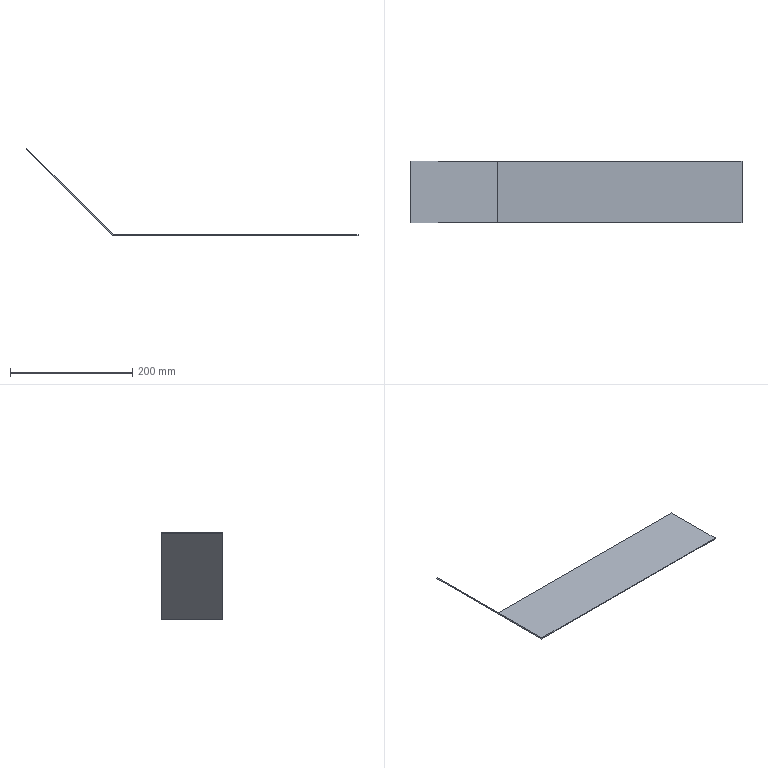Part | STEP file | Mirror Velcro | 1 solid | 8 faces | box 542.128 x 100 x 143.128 mm | volume 120000 mm3 | plane 8
STEP:
#1=CARTESIAN_POINT('',(0.,0.,0.));
#2=DIRECTION('',(0.,0.,1.));
#3=DIRECTION('',(1.,0.,0.));
#4=AXIS2_PLACEMENT_3D('',#1,#2,#3);
#5=CARTESIAN_POINT('',(-0.4142,-50.,-1.));
#6=VERTEX_POINT('',#5);
#7=CARTESIAN_POINT('',(400.,-50.,-1.));
#8=VERTEX_POINT('',#7);
#9=CARTESIAN_POINT('',(0.,-50.,-1.));
#10=DIRECTION('',(1.,0.,0.));
#11=VECTOR('',#10,1.);
#12=LINE('',#9,#11);
#13=CARTESIAN_POINT('',(0.,50.,-1.));
#14=DIRECTION('',(0.,0.,1.));
#15=DIRECTION('',(-1.,0.,0.));
#16=AXIS2_PLACEMENT_3D('',#13,#14,#15);
#17=PLANE('',#16);
#18=CARTESIAN_POINT('',(0.,100.));
#19=DIRECTION('',(-1.,0.));
#20=VECTOR('',#19,1.);
#21=LINE('',#18,#20);
#22=(GEOMETRIC_REPRESENTATION_CONTEXT(2)PARAMETRIC_REPRESENTATION_CONTEXT()REPRESENTATION_CONTEXT('',''));
#23=DEFINITIONAL_REPRESENTATION('',(#21),#22);
#24=PCURVE('',#17,#23);
#25=CARTESIAN_POINT('',(0.,-50.,0.));
#26=DIRECTION('',(0.,-1.,0.));
#27=DIRECTION('',(-1.,0.,0.));
#28=AXIS2_PLACEMENT_3D('',#25,#26,#27);
#29=PLANE('',#28);
#30=CARTESIAN_POINT('',(0.,1.));
#31=DIRECTION('',(-1.,0.));
#32=VECTOR('',#31,1.);
#33=LINE('',#30,#32);
#34=(GEOMETRIC_REPRESENTATION_CONTEXT(2)PARAMETRIC_REPRESENTATION_CONTEXT()REPRESENTATION_CONTEXT('',''));
#35=DEFINITIONAL_REPRESENTATION('',(#33),#34);
#36=PCURVE('',#29,#35);
#37=SURFACE_CURVE('',#12,(#24,#36),.PCURVE_S1.);
#38=EDGE_CURVE('',#6,#8,#37,.T.);
#39=ORIENTED_EDGE('',*,*,#38,.F.);
#40=CARTESIAN_POINT('',(-0.4142,50.,-1.));
#41=VERTEX_POINT('',#40);
#42=CARTESIAN_POINT('',(-0.4142,50.,-1.));
#43=DIRECTION('',(0.,-1.,0.));
#44=VECTOR('',#43,1.);
#45=LINE('',#42,#44);
#46=CARTESIAN_POINT('',(0.4142,0.));
#47=DIRECTION('',(0.,1.));
#48=VECTOR('',#47,1.);
#49=LINE('',#46,#48);
#50=(GEOMETRIC_REPRESENTATION_CONTEXT(2)PARAMETRIC_REPRESENTATION_CONTEXT()REPRESENTATION_CONTEXT('',''));
#51=DEFINITIONAL_REPRESENTATION('',(#49),#50);
#52=PCURVE('',#17,#51);
#53=CARTESIAN_POINT('',(-142.128,50.,140.714));
#54=DIRECTION('',(0.7071,0.,0.7071));
#55=DIRECTION('',(-0.7071,0.,0.7071));
#56=AXIS2_PLACEMENT_3D('',#53,#54,#55);
#57=PLANE('',#56);
#58=CARTESIAN_POINT('',(-200.414,0.));
#59=DIRECTION('',(0.,1.));
#60=VECTOR('',#59,1.);
#61=LINE('',#58,#60);
#62=(GEOMETRIC_REPRESENTATION_CONTEXT(2)PARAMETRIC_REPRESENTATION_CONTEXT()REPRESENTATION_CONTEXT('',''));
#63=DEFINITIONAL_REPRESENTATION('',(#61),#62);
#64=PCURVE('',#57,#63);
#65=SURFACE_CURVE('',#45,(#52,#64),.PCURVE_S1.);
#66=EDGE_CURVE('',#41,#6,#65,.T.);
#67=ORIENTED_EDGE('',*,*,#66,.F.);
#68=CARTESIAN_POINT('',(400.,50.,-1.));
#69=VERTEX_POINT('',#68);
#70=CARTESIAN_POINT('',(0.,50.,-1.));
#71=DIRECTION('',(1.,0.,0.));
#72=VECTOR('',#71,1.);
#73=LINE('',#70,#72);
#74=CARTESIAN_POINT('',(0.,0.));
#75=DIRECTION('',(-1.,0.));
#76=VECTOR('',#75,1.);
#77=LINE('',#74,#76);
#78=(GEOMETRIC_REPRESENTATION_CONTEXT(2)PARAMETRIC_REPRESENTATION_CONTEXT()REPRESENTATION_CONTEXT('',''));
#79=DEFINITIONAL_REPRESENTATION('',(#77),#78);
#80=PCURVE('',#17,#79);
#81=CARTESIAN_POINT('',(0.,50.,0.));
#82=DIRECTION('',(0.,-1.,0.));
#83=DIRECTION('',(-1.,0.,0.));
#84=AXIS2_PLACEMENT_3D('',#81,#82,#83);
#85=PLANE('',#84);
#86=CARTESIAN_POINT('',(0.,1.));
#87=DIRECTION('',(-1.,0.));
#88=VECTOR('',#87,1.);
#89=LINE('',#86,#88);
#90=(GEOMETRIC_REPRESENTATION_CONTEXT(2)PARAMETRIC_REPRESENTATION_CONTEXT()REPRESENTATION_CONTEXT('',''));
#91=DEFINITIONAL_REPRESENTATION('',(#89),#90);
#92=PCURVE('',#85,#91);
#93=SURFACE_CURVE('',#73,(#80,#92),.PCURVE_S1.);
#94=EDGE_CURVE('',#41,#69,#93,.T.);
#95=ORIENTED_EDGE('',*,*,#94,.T.);
#96=CARTESIAN_POINT('',(400.,50.,-1.));
#97=DIRECTION('',(0.,-1.,0.));
#98=VECTOR('',#97,1.);
#99=LINE('',#96,#98);
#100=CARTESIAN_POINT('',(-400.,0.));
#101=DIRECTION('',(0.,1.));
#102=VECTOR('',#101,1.);
#103=LINE('',#100,#102);
#104=(GEOMETRIC_REPRESENTATION_CONTEXT(2)PARAMETRIC_REPRESENTATION_CONTEXT()REPRESENTATION_CONTEXT('',''));
#105=DEFINITIONAL_REPRESENTATION('',(#103),#104);
#106=PCURVE('',#17,#105);
#107=CARTESIAN_POINT('',(400.,50.,1.));
#108=DIRECTION('',(1.,0.,0.));
#109=DIRECTION('',(0.,0.,1.));
#110=AXIS2_PLACEMENT_3D('',#107,#108,#109);
#111=PLANE('',#110);
#112=CARTESIAN_POINT('',(-2.,0.));
#113=DIRECTION('',(0.,1.));
#114=VECTOR('',#113,1.);
#115=LINE('',#112,#114);
#116=(GEOMETRIC_REPRESENTATION_CONTEXT(2)PARAMETRIC_REPRESENTATION_CONTEXT()REPRESENTATION_CONTEXT('',''));
#117=DEFINITIONAL_REPRESENTATION('',(#115),#116);
#118=PCURVE('',#111,#117);
#119=SURFACE_CURVE('',#99,(#106,#118),.PCURVE_S1.);
#120=EDGE_CURVE('',#69,#8,#119,.T.);
#121=ORIENTED_EDGE('',*,*,#120,.T.);
#122=EDGE_LOOP('',(#39,#67,#95,#121));
#123=FACE_BOUND('',#122,.T.);
#124=ADVANCED_FACE('',(#123),#17,.F.);
#125=CARTESIAN_POINT('',(400.,-50.,1.));
#126=VERTEX_POINT('',#125);
#127=CARTESIAN_POINT('',(400.,-50.,1.));
#128=DIRECTION('',(0.,0.,-1.));
#129=VECTOR('',#128,1.);
#130=LINE('',#127,#129);
#131=CARTESIAN_POINT('',(0.,100.));
#132=DIRECTION('',(-1.,0.));
#133=VECTOR('',#132,1.);
#134=LINE('',#131,#133);
#135=(GEOMETRIC_REPRESENTATION_CONTEXT(2)PARAMETRIC_REPRESENTATION_CONTEXT()REPRESENTATION_CONTEXT('',''));
#136=DEFINITIONAL_REPRESENTATION('',(#134),#135);
#137=PCURVE('',#111,#136);
#138=CARTESIAN_POINT('',(-400.,-1.));
#139=DIRECTION('',(0.,1.));
#140=VECTOR('',#139,1.);
#141=LINE('',#138,#140);
#142=(GEOMETRIC_REPRESENTATION_CONTEXT(2)PARAMETRIC_REPRESENTATION_CONTEXT()REPRESENTATION_CONTEXT('',''));
#143=DEFINITIONAL_REPRESENTATION('',(#141),#142);
#144=PCURVE('',#29,#143);
#145=SURFACE_CURVE('',#130,(#137,#144),.PCURVE_S1.);
#146=EDGE_CURVE('',#126,#8,#145,.T.);
#147=ORIENTED_EDGE('',*,*,#146,.T.);
#148=ORIENTED_EDGE('',*,*,#120,.F.);
#149=CARTESIAN_POINT('',(400.,50.,1.));
#150=VERTEX_POINT('',#149);
#151=CARTESIAN_POINT('',(400.,50.,1.));
#152=DIRECTION('',(0.,0.,-1.));
#153=VECTOR('',#152,1.);
#154=LINE('',#151,#153);
#155=CARTESIAN_POINT('',(0.,0.));
#156=DIRECTION('',(-1.,0.));
#157=VECTOR('',#156,1.);
#158=LINE('',#155,#157);
#159=(GEOMETRIC_REPRESENTATION_CONTEXT(2)PARAMETRIC_REPRESENTATION_CONTEXT()REPRESENTATION_CONTEXT('',''));
#160=DEFINITIONAL_REPRESENTATION('',(#158),#159);
#161=PCURVE('',#111,#160);
#162=CARTESIAN_POINT('',(-400.,-1.));
#163=DIRECTION('',(0.,1.));
#164=VECTOR('',#163,1.);
#165=LINE('',#162,#164);
#166=(GEOMETRIC_REPRESENTATION_CONTEXT(2)PARAMETRIC_REPRESENTATION_CONTEXT()REPRESENTATION_CONTEXT('',''));
#167=DEFINITIONAL_REPRESENTATION('',(#165),#166);
#168=PCURVE('',#85,#167);
#169=SURFACE_CURVE('',#154,(#161,#168),.PCURVE_S1.);
#170=EDGE_CURVE('',#150,#69,#169,.T.);
#171=ORIENTED_EDGE('',*,*,#170,.F.);
#172=CARTESIAN_POINT('',(400.,50.,1.));
#173=DIRECTION('',(0.,-1.,0.));
#174=VECTOR('',#173,1.);
#175=LINE('',#172,#174);
#176=CARTESIAN_POINT('',(0.,0.));
#177=DIRECTION('',(0.,1.));
#178=VECTOR('',#177,1.);
#179=LINE('',#176,#178);
#180=(GEOMETRIC_REPRESENTATION_CONTEXT(2)PARAMETRIC_REPRESENTATION_CONTEXT()REPRESENTATION_CONTEXT('',''));
#181=DEFINITIONAL_REPRESENTATION('',(#179),#180);
#182=PCURVE('',#111,#181);
#183=CARTESIAN_POINT('',(0.,50.,1.));
#184=DIRECTION('',(0.,0.,1.));
#185=DIRECTION('',(-1.,0.,0.));
#186=AXIS2_PLACEMENT_3D('',#183,#184,#185);
#187=PLANE('',#186);
#188=CARTESIAN_POINT('',(-400.,0.));
#189=DIRECTION('',(0.,1.));
#190=VECTOR('',#189,1.);
#191=LINE('',#188,#190);
#192=(GEOMETRIC_REPRESENTATION_CONTEXT(2)PARAMETRIC_REPRESENTATION_CONTEXT()REPRESENTATION_CONTEXT('',''));
#193=DEFINITIONAL_REPRESENTATION('',(#191),#192);
#194=PCURVE('',#187,#193);
#195=SURFACE_CURVE('',#175,(#182,#194),.PCURVE_S1.);
#196=EDGE_CURVE('',#150,#126,#195,.T.);
#197=ORIENTED_EDGE('',*,*,#196,.T.);
#198=EDGE_LOOP('',(#147,#148,#171,#197));
#199=FACE_BOUND('',#198,.T.);
#200=ADVANCED_FACE('',(#199),#111,.T.);
#201=CARTESIAN_POINT('',(0.4142,-50.,1.));
#202=VERTEX_POINT('',#201);
#203=CARTESIAN_POINT('',(0.,-50.,1.));
#204=DIRECTION('',(1.,0.,0.));
#205=VECTOR('',#204,1.);
#206=LINE('',#203,#205);
#207=CARTESIAN_POINT('',(0.,100.));
#208=DIRECTION('',(-1.,0.));
#209=VECTOR('',#208,1.);
#210=LINE('',#207,#209);
#211=(GEOMETRIC_REPRESENTATION_CONTEXT(2)PARAMETRIC_REPRESENTATION_CONTEXT()REPRESENTATION_CONTEXT('',''));
#212=DEFINITIONAL_REPRESENTATION('',(#210),#211);
#213=PCURVE('',#187,#212);
#214=CARTESIAN_POINT('',(0.,-1.));
#215=DIRECTION('',(-1.,0.));
#216=VECTOR('',#215,1.);
#217=LINE('',#214,#216);
#218=(GEOMETRIC_REPRESENTATION_CONTEXT(2)PARAMETRIC_REPRESENTATION_CONTEXT()REPRESENTATION_CONTEXT('',''));
#219=DEFINITIONAL_REPRESENTATION('',(#217),#218);
#220=PCURVE('',#29,#219);
#221=SURFACE_CURVE('',#206,(#213,#220),.PCURVE_S1.);
#222=EDGE_CURVE('',#202,#126,#221,.T.);
#223=ORIENTED_EDGE('',*,*,#222,.T.);
#224=ORIENTED_EDGE('',*,*,#196,.F.);
#225=CARTESIAN_POINT('',(0.4142,50.,1.));
#226=VERTEX_POINT('',#225);
#227=CARTESIAN_POINT('',(0.,50.,1.));
#228=DIRECTION('',(1.,0.,0.));
#229=VECTOR('',#228,1.);
#230=LINE('',#227,#229);
#231=CARTESIAN_POINT('',(0.,0.));
#232=DIRECTION('',(-1.,0.));
#233=VECTOR('',#232,1.);
#234=LINE('',#231,#233);
#235=(GEOMETRIC_REPRESENTATION_CONTEXT(2)PARAMETRIC_REPRESENTATION_CONTEXT()REPRESENTATION_CONTEXT('',''));
#236=DEFINITIONAL_REPRESENTATION('',(#234),#235);
#237=PCURVE('',#187,#236);
#238=CARTESIAN_POINT('',(0.,-1.));
#239=DIRECTION('',(-1.,0.));
#240=VECTOR('',#239,1.);
#241=LINE('',#238,#240);
#242=(GEOMETRIC_REPRESENTATION_CONTEXT(2)PARAMETRIC_REPRESENTATION_CONTEXT()REPRESENTATION_CONTEXT('',''));
#243=DEFINITIONAL_REPRESENTATION('',(#241),#242);
#244=PCURVE('',#85,#243);
#245=SURFACE_CURVE('',#230,(#237,#244),.PCURVE_S1.);
#246=EDGE_CURVE('',#226,#150,#245,.T.);
#247=ORIENTED_EDGE('',*,*,#246,.F.);
#248=CARTESIAN_POINT('',(0.4142,50.,1.));
#249=DIRECTION('',(0.,-1.,0.));
#250=VECTOR('',#249,1.);
#251=LINE('',#248,#250);
#252=CARTESIAN_POINT('',(-0.4142,0.));
#253=DIRECTION('',(0.,1.));
#254=VECTOR('',#253,1.);
#255=LINE('',#252,#254);
#256=(GEOMETRIC_REPRESENTATION_CONTEXT(2)PARAMETRIC_REPRESENTATION_CONTEXT()REPRESENTATION_CONTEXT('',''));
#257=DEFINITIONAL_REPRESENTATION('',(#255),#256);
#258=PCURVE('',#187,#257);
#259=CARTESIAN_POINT('',(-140.714,50.,142.128));
#260=DIRECTION('',(0.7071,0.,0.7071));
#261=DIRECTION('',(-0.7071,0.,0.7071));
#262=AXIS2_PLACEMENT_3D('',#259,#260,#261);
#263=PLANE('',#262);
#264=CARTESIAN_POINT('',(-199.586,0.));
#265=DIRECTION('',(0.,1.));
#266=VECTOR('',#265,1.);
#267=LINE('',#264,#266);
#268=(GEOMETRIC_REPRESENTATION_CONTEXT(2)PARAMETRIC_REPRESENTATION_CONTEXT()REPRESENTATION_CONTEXT('',''));
#269=DEFINITIONAL_REPRESENTATION('',(#267),#268);
#270=PCURVE('',#263,#269);
#271=SURFACE_CURVE('',#251,(#258,#270),.PCURVE_S1.);
#272=EDGE_CURVE('',#226,#202,#271,.T.);
#273=ORIENTED_EDGE('',*,*,#272,.T.);
#274=EDGE_LOOP('',(#223,#224,#247,#273));
#275=FACE_BOUND('',#274,.T.);
#276=ADVANCED_FACE('',(#275),#187,.T.);
#277=CARTESIAN_POINT('',(-140.714,-50.,142.128));
#278=VERTEX_POINT('',#277);
#279=CARTESIAN_POINT('',(-140.714,-50.,142.128));
#280=DIRECTION('',(0.7071,0.,-0.7071));
#281=VECTOR('',#280,1.);
#282=LINE('',#279,#281);
#283=CARTESIAN_POINT('',(0.,100.));
#284=DIRECTION('',(-1.,0.));
#285=VECTOR('',#284,1.);
#286=LINE('',#283,#285);
#287=(GEOMETRIC_REPRESENTATION_CONTEXT(2)PARAMETRIC_REPRESENTATION_CONTEXT()REPRESENTATION_CONTEXT('',''));
#288=DEFINITIONAL_REPRESENTATION('',(#286),#287);
#289=PCURVE('',#263,#288);
#290=CARTESIAN_POINT('',(140.714,-142.128));
#291=DIRECTION('',(-0.7071,0.7071));
#292=VECTOR('',#291,1.);
#293=LINE('',#290,#292);
#294=(GEOMETRIC_REPRESENTATION_CONTEXT(2)PARAMETRIC_REPRESENTATION_CONTEXT()REPRESENTATION_CONTEXT('',''));
#295=DEFINITIONAL_REPRESENTATION('',(#293),#294);
#296=PCURVE('',#29,#295);
#297=SURFACE_CURVE('',#282,(#289,#296),.PCURVE_S1.);
#298=EDGE_CURVE('',#278,#202,#297,.T.);
#299=ORIENTED_EDGE('',*,*,#298,.T.);
#300=ORIENTED_EDGE('',*,*,#272,.F.);
#301=CARTESIAN_POINT('',(-140.714,50.,142.128));
#302=VERTEX_POINT('',#301);
#303=CARTESIAN_POINT('',(-140.714,50.,142.128));
#304=DIRECTION('',(0.7071,0.,-0.7071));
#305=VECTOR('',#304,1.);
#306=LINE('',#303,#305);
#307=CARTESIAN_POINT('',(0.,0.));
#308=DIRECTION('',(-1.,0.));
#309=VECTOR('',#308,1.);
#310=LINE('',#307,#309);
#311=(GEOMETRIC_REPRESENTATION_CONTEXT(2)PARAMETRIC_REPRESENTATION_CONTEXT()REPRESENTATION_CONTEXT('',''));
#312=DEFINITIONAL_REPRESENTATION('',(#310),#311);
#313=PCURVE('',#263,#312);
#314=CARTESIAN_POINT('',(140.714,-142.128));
#315=DIRECTION('',(-0.7071,0.7071));
#316=VECTOR('',#315,1.);
#317=LINE('',#314,#316);
#318=(GEOMETRIC_REPRESENTATION_CONTEXT(2)PARAMETRIC_REPRESENTATION_CONTEXT()REPRESENTATION_CONTEXT('',''));
#319=DEFINITIONAL_REPRESENTATION('',(#317),#318);
#320=PCURVE('',#85,#319);
#321=SURFACE_CURVE('',#306,(#313,#320),.PCURVE_S1.);
#322=EDGE_CURVE('',#302,#226,#321,.T.);
#323=ORIENTED_EDGE('',*,*,#322,.F.);
#324=CARTESIAN_POINT('',(-140.714,50.,142.128));
#325=DIRECTION('',(0.,-1.,0.));
#326=VECTOR('',#325,1.);
#327=LINE('',#324,#326);
#328=CARTESIAN_POINT('',(0.,0.));
#329=DIRECTION('',(0.,1.));
#330=VECTOR('',#329,1.);
#331=LINE('',#328,#330);
#332=(GEOMETRIC_REPRESENTATION_CONTEXT(2)PARAMETRIC_REPRESENTATION_CONTEXT()REPRESENTATION_CONTEXT('',''));
#333=DEFINITIONAL_REPRESENTATION('',(#331),#332);
#334=PCURVE('',#263,#333);
#335=CARTESIAN_POINT('',(-142.128,50.,140.714));
#336=DIRECTION('',(-0.7071,0.,0.7071));
#337=DIRECTION('',(-0.7071,0.,-0.7071));
#338=AXIS2_PLACEMENT_3D('',#335,#336,#337);
#339=PLANE('',#338);
#340=CARTESIAN_POINT('',(-2.,0.));
#341=DIRECTION('',(0.,1.));
#342=VECTOR('',#341,1.);
#343=LINE('',#340,#342);
#344=(GEOMETRIC_REPRESENTATION_CONTEXT(2)PARAMETRIC_REPRESENTATION_CONTEXT()REPRESENTATION_CONTEXT('',''));
#345=DEFINITIONAL_REPRESENTATION('',(#343),#344);
#346=PCURVE('',#339,#345);
#347=SURFACE_CURVE('',#327,(#334,#346),.PCURVE_S1.);
#348=EDGE_CURVE('',#302,#278,#347,.T.);
#349=ORIENTED_EDGE('',*,*,#348,.T.);
#350=EDGE_LOOP('',(#299,#300,#323,#349));
#351=FACE_BOUND('',#350,.T.);
#352=ADVANCED_FACE('',(#351),#263,.T.);
#353=CARTESIAN_POINT('',(-142.128,-50.,140.714));
#354=VERTEX_POINT('',#353);
#355=CARTESIAN_POINT('',(-142.128,-50.,140.714));
#356=DIRECTION('',(0.7071,0.,0.7071));
#357=VECTOR('',#356,1.);
#358=LINE('',#355,#357);
#359=CARTESIAN_POINT('',(0.,100.));
#360=DIRECTION('',(-1.,0.));
#361=VECTOR('',#360,1.);
#362=LINE('',#359,#361);
#363=(GEOMETRIC_REPRESENTATION_CONTEXT(2)PARAMETRIC_REPRESENTATION_CONTEXT()REPRESENTATION_CONTEXT('',''));
#364=DEFINITIONAL_REPRESENTATION('',(#362),#363);
#365=PCURVE('',#339,#364);
#366=CARTESIAN_POINT('',(142.128,-140.714));
#367=DIRECTION('',(-0.7071,-0.7071));
#368=VECTOR('',#367,1.);
#369=LINE('',#366,#368);
#370=(GEOMETRIC_REPRESENTATION_CONTEXT(2)PARAMETRIC_REPRESENTATION_CONTEXT()REPRESENTATION_CONTEXT('',''));
#371=DEFINITIONAL_REPRESENTATION('',(#369),#370);
#372=PCURVE('',#29,#371);
#373=SURFACE_CURVE('',#358,(#365,#372),.PCURVE_S1.);
#374=EDGE_CURVE('',#354,#278,#373,.T.);
#375=ORIENTED_EDGE('',*,*,#374,.T.);
#376=ORIENTED_EDGE('',*,*,#348,.F.);
#377=CARTESIAN_POINT('',(-142.128,50.,140.714));
#378=VERTEX_POINT('',#377);
#379=CARTESIAN_POINT('',(-142.128,50.,140.714));
#380=DIRECTION('',(0.7071,0.,0.7071));
#381=VECTOR('',#380,1.);
#382=LINE('',#379,#381);
#383=CARTESIAN_POINT('',(0.,0.));
#384=DIRECTION('',(-1.,0.));
#385=VECTOR('',#384,1.);
#386=LINE('',#383,#385);
#387=(GEOMETRIC_REPRESENTATION_CONTEXT(2)PARAMETRIC_REPRESENTATION_CONTEXT()REPRESENTATION_CONTEXT('',''));
#388=DEFINITIONAL_REPRESENTATION('',(#386),#387);
#389=PCURVE('',#339,#388);
#390=CARTESIAN_POINT('',(142.128,-140.714));
#391=DIRECTION('',(-0.7071,-0.7071));
#392=VECTOR('',#391,1.);
#393=LINE('',#390,#392);
#394=(GEOMETRIC_REPRESENTATION_CONTEXT(2)PARAMETRIC_REPRESENTATION_CONTEXT()REPRESENTATION_CONTEXT('',''));
#395=DEFINITIONAL_REPRESENTATION('',(#393),#394);
#396=PCURVE('',#85,#395);
#397=SURFACE_CURVE('',#382,(#389,#396),.PCURVE_S1.);
#398=EDGE_CURVE('',#378,#302,#397,.T.);
#399=ORIENTED_EDGE('',*,*,#398,.F.);
#400=CARTESIAN_POINT('',(-142.128,50.,140.714));
#401=DIRECTION('',(0.,-1.,0.));
#402=VECTOR('',#401,1.);
#403=LINE('',#400,#402);
#404=CARTESIAN_POINT('',(0.,0.));
#405=DIRECTION('',(0.,1.));
#406=VECTOR('',#405,1.);
#407=LINE('',#404,#406);
#408=(GEOMETRIC_REPRESENTATION_CONTEXT(2)PARAMETRIC_REPRESENTATION_CONTEXT()REPRESENTATION_CONTEXT('',''));
#409=DEFINITIONAL_REPRESENTATION('',(#407),#408);
#410=PCURVE('',#339,#409);
#411=CARTESIAN_POINT('',(0.,0.));
#412=DIRECTION('',(0.,1.));
#413=VECTOR('',#412,1.);
#414=LINE('',#411,#413);
#415=(GEOMETRIC_REPRESENTATION_CONTEXT(2)PARAMETRIC_REPRESENTATION_CONTEXT()REPRESENTATION_CONTEXT('',''));
#416=DEFINITIONAL_REPRESENTATION('',(#414),#415);
#417=PCURVE('',#57,#416);
#418=SURFACE_CURVE('',#403,(#410,#417),.PCURVE_S1.);
#419=EDGE_CURVE('',#378,#354,#418,.T.);
#420=ORIENTED_EDGE('',*,*,#419,.T.);
#421=EDGE_LOOP('',(#375,#376,#399,#420));
#422=FACE_BOUND('',#421,.T.);
#423=ADVANCED_FACE('',(#422),#339,.T.);
#424=CARTESIAN_POINT('',(-142.128,-50.,140.714));
#425=DIRECTION('',(0.7071,0.,-0.7071));
#426=VECTOR('',#425,1.);
#427=LINE('',#424,#426);
#428=CARTESIAN_POINT('',(0.,100.));
#429=DIRECTION('',(-1.,0.));
#430=VECTOR('',#429,1.);
#431=LINE('',#428,#430);
#432=(GEOMETRIC_REPRESENTATION_CONTEXT(2)PARAMETRIC_REPRESENTATION_CONTEXT()REPRESENTATION_CONTEXT('',''));
#433=DEFINITIONAL_REPRESENTATION('',(#431),#432);
#434=PCURVE('',#57,#433);
#435=CARTESIAN_POINT('',(142.128,-140.714));
#436=DIRECTION('',(-0.7071,0.7071));
#437=VECTOR('',#436,1.);
#438=LINE('',#435,#437);
#439=(GEOMETRIC_REPRESENTATION_CONTEXT(2)PARAMETRIC_REPRESENTATION_CONTEXT()REPRESENTATION_CONTEXT('',''));
#440=DEFINITIONAL_REPRESENTATION('',(#438),#439);
#441=PCURVE('',#29,#440);
#442=SURFACE_CURVE('',#427,(#434,#441),.PCURVE_S1.);
#443=EDGE_CURVE('',#354,#6,#442,.T.);
#444=ORIENTED_EDGE('',*,*,#443,.F.);
#445=ORIENTED_EDGE('',*,*,#419,.F.);
#446=CARTESIAN_POINT('',(-142.128,50.,140.714));
#447=DIRECTION('',(0.7071,0.,-0.7071));
#448=VECTOR('',#447,1.);
#449=LINE('',#446,#448);
#450=CARTESIAN_POINT('',(0.,0.));
#451=DIRECTION('',(-1.,0.));
#452=VECTOR('',#451,1.);
#453=LINE('',#450,#452);
#454=(GEOMETRIC_REPRESENTATION_CONTEXT(2)PARAMETRIC_REPRESENTATION_CONTEXT()REPRESENTATION_CONTEXT('',''));
#455=DEFINITIONAL_REPRESENTATION('',(#453),#454);
#456=PCURVE('',#57,#455);
#457=CARTESIAN_POINT('',(142.128,-140.714));
#458=DIRECTION('',(-0.7071,0.7071));
#459=VECTOR('',#458,1.);
#460=LINE('',#457,#459);
#461=(GEOMETRIC_REPRESENTATION_CONTEXT(2)PARAMETRIC_REPRESENTATION_CONTEXT()REPRESENTATION_CONTEXT('',''));
#462=DEFINITIONAL_REPRESENTATION('',(#460),#461);
#463=PCURVE('',#85,#462);
#464=SURFACE_CURVE('',#449,(#456,#463),.PCURVE_S1.);
#465=EDGE_CURVE('',#378,#41,#464,.T.);
#466=ORIENTED_EDGE('',*,*,#465,.T.);
#467=ORIENTED_EDGE('',*,*,#66,.T.);
#468=EDGE_LOOP('',(#444,#445,#466,#467));
#469=FACE_BOUND('',#468,.T.);
#470=ADVANCED_FACE('',(#469),#57,.F.);
#471=ORIENTED_EDGE('',*,*,#94,.F.);
#472=ORIENTED_EDGE('',*,*,#465,.F.);
#473=ORIENTED_EDGE('',*,*,#398,.T.);
#474=ORIENTED_EDGE('',*,*,#322,.T.);
#475=ORIENTED_EDGE('',*,*,#246,.T.);
#476=ORIENTED_EDGE('',*,*,#170,.T.);
#477=EDGE_LOOP('',(#471,#472,#473,#474,#475,#476));
#478=FACE_BOUND('',#477,.T.);
#479=ADVANCED_FACE('',(#478),#85,.F.);
#480=ORIENTED_EDGE('',*,*,#38,.T.);
#481=ORIENTED_EDGE('',*,*,#146,.F.);
#482=ORIENTED_EDGE('',*,*,#222,.F.);
#483=ORIENTED_EDGE('',*,*,#298,.F.);
#484=ORIENTED_EDGE('',*,*,#374,.F.);
#485=ORIENTED_EDGE('',*,*,#443,.T.);
#486=EDGE_LOOP('',(#480,#481,#482,#483,#484,#485));
#487=FACE_BOUND('',#486,.T.);
#488=ADVANCED_FACE('',(#487),#29,.T.);
#489=CLOSED_SHELL('',(#124,#200,#276,#352,#423,#470,#479,#488));
#490=MANIFOLD_SOLID_BREP('',#489);
#491=(LENGTH_UNIT()NAMED_UNIT(*)SI_UNIT(.MILLI.,.METRE.));
#492=UNCERTAINTY_MEASURE_WITH_UNIT(LENGTH_MEASURE(0.0000001),#491,'','');
#493=(NAMED_UNIT(*)PLANE_ANGLE_UNIT()SI_UNIT($,.RADIAN.));
#494=(NAMED_UNIT(*)SI_UNIT($,.STERADIAN.)SOLID_ANGLE_UNIT());
#495=(GEOMETRIC_REPRESENTATION_CONTEXT(3)GLOBAL_UNCERTAINTY_ASSIGNED_CONTEXT((#492))GLOBAL_UNIT_ASSIGNED_CONTEXT((#491,#493,#494))REPRESENTATION_CONTEXT('',''));
#496=ADVANCED_BREP_SHAPE_REPRESENTATION('',(#4,#490),#495);